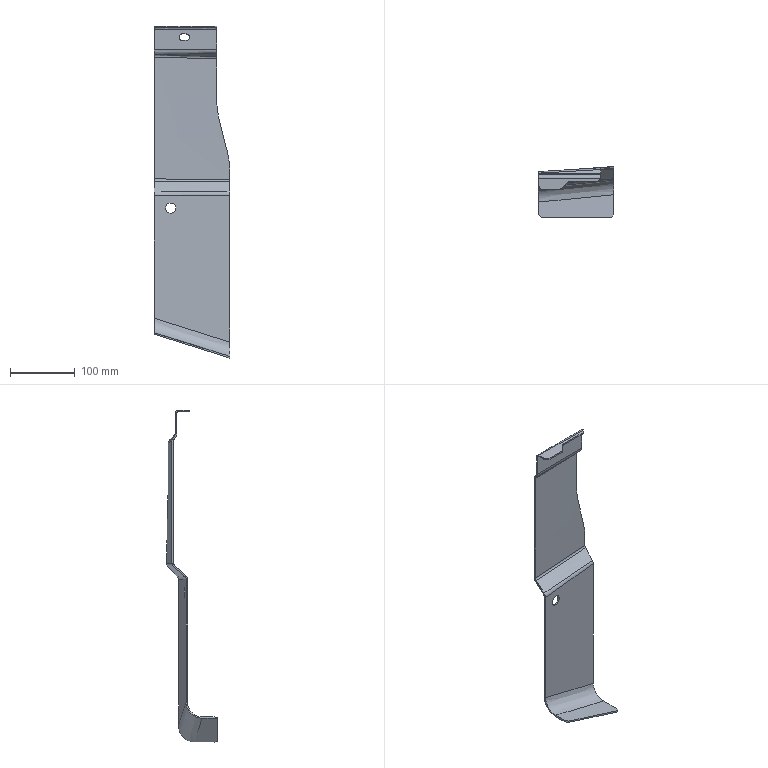Part | SolidWorks | features BaseBody 1 | 1 solid | 57 faces | box 116.807 x 78.32 x 514.503 mm | volume 142015 mm3 | spline 28 | plane 21 | cylinder 8 | commonest cylinder face diameters 10 x4 16 x2 200 x2